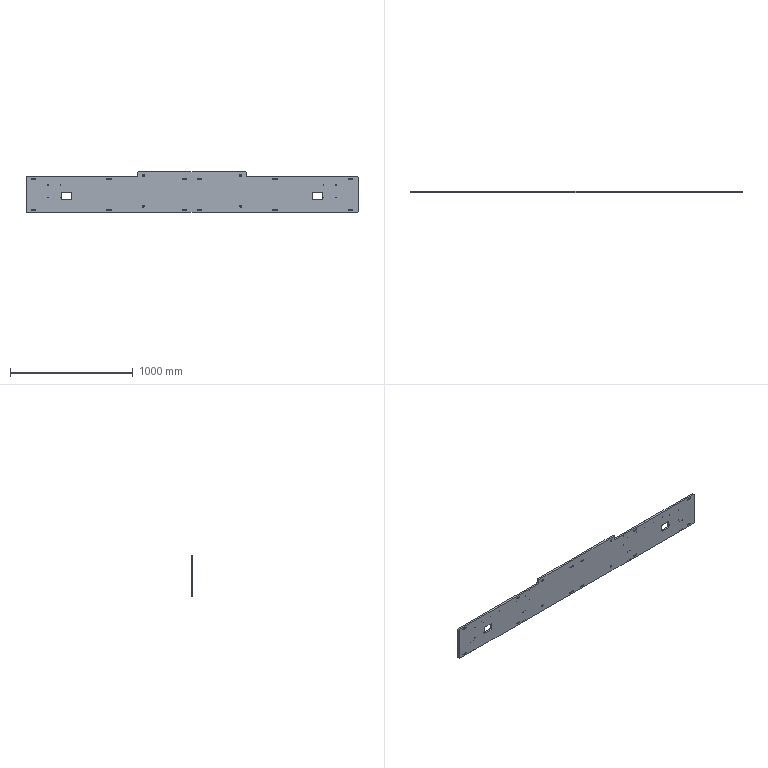Part | SolidWorks | features HoleWzd 7, ICE 4, Chamfer 1, Extrusion 1, Fillet 1, PLine 1 | 1 solid | 385 faces | box 2700 x 15 x 330 mm | volume 12065498 mm3 | cylinder 242 | cone 96 | plane 47 | commonest cylinder face diameters 3.3 x64 6.8 x64 4.2 x32 9 x24 15 x24 10 x8